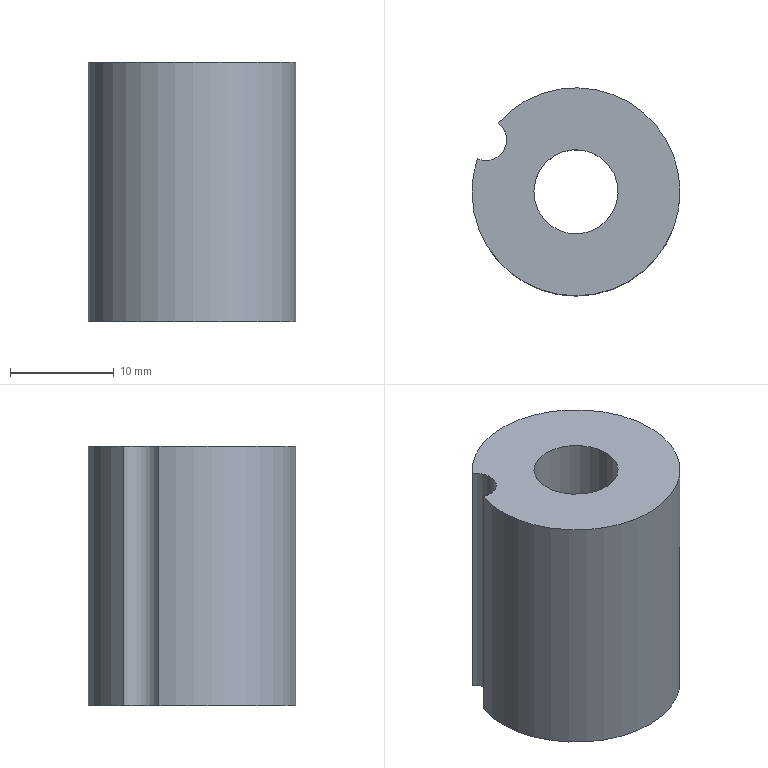Part | NX | features solid 2 | 1 solid | 7 faces | box 20 x 20 x 25 mm | volume 5172 mm3 | cylinder 4 | plane 3 | commonest cylinder face diameters 4 x1 8.1 x1 12.6 x1 20 x1
STEP:
#1=CARTESIAN_POINT('',(-312.495,434.194,24.));
#2=VERTEX_POINT('',#1);
#3=CARTESIAN_POINT('',(-312.495,434.194,49.));
#4=VERTEX_POINT('',#3);
#5=CARTESIAN_POINT('',(-312.495,434.194,36.5));
#6=DIRECTION('',(0.,0.,1.));
#7=VECTOR('',#6,1000.);
#8=LINE('',#5,#7);
#9=EDGE_CURVE('',#2,#4,#8,.T.);
#10=ORIENTED_EDGE('',*,*,#9,.T.);
#11=CARTESIAN_POINT('',(-314.485,430.747,49.));
#12=VERTEX_POINT('',#11);
#13=CARTESIAN_POINT('',(-305.003,427.57,49.));
#14=DIRECTION('',(0.,0.,-1.));
#15=DIRECTION('',(-0.866,0.5,0.));
#16=AXIS2_PLACEMENT_3D('',#13,#14,#15);
#17=CIRCLE('',#16,10.);
#18=EDGE_CURVE('',#4,#12,#17,.T.);
#19=ORIENTED_EDGE('',*,*,#18,.T.);
#20=CARTESIAN_POINT('',(-314.485,430.747,24.));
#21=VERTEX_POINT('',#20);
#22=CARTESIAN_POINT('',(-314.485,430.747,36.5));
#23=DIRECTION('',(0.,0.,1.));
#24=VECTOR('',#23,1000.);
#25=LINE('',#22,#24);
#26=EDGE_CURVE('',#12,#21,#25,.F.);
#27=ORIENTED_EDGE('',*,*,#26,.T.);
#28=CARTESIAN_POINT('',(-305.003,427.57,24.));
#29=DIRECTION('',(0.,0.,-1.));
#30=DIRECTION('',(-0.866,0.5,0.));
#31=AXIS2_PLACEMENT_3D('',#28,#29,#30);
#32=CIRCLE('',#31,10.);
#33=EDGE_CURVE('',#2,#21,#32,.T.);
#34=ORIENTED_EDGE('',*,*,#33,.F.);
#35=EDGE_LOOP('',(#10,#19,#27,#34));
#36=FACE_BOUND('',#35,.T.);
#37=CARTESIAN_POINT('',(-305.003,427.57,24.));
#38=DIRECTION('',(0.,0.,1.));
#39=DIRECTION('',(-0.866,0.5,0.));
#40=AXIS2_PLACEMENT_3D('',#37,#38,#39);
#41=CYLINDRICAL_SURFACE('',#40,10.);
#42=ADVANCED_FACE('',(#36),#41,.T.);
#43=CARTESIAN_POINT('',(-310.459,430.72,24.));
#44=VERTEX_POINT('',#43);
#45=CARTESIAN_POINT('',(-305.003,427.57,24.));
#46=DIRECTION('',(0.,0.,-1.));
#47=DIRECTION('',(-0.866,0.5,0.));
#48=AXIS2_PLACEMENT_3D('',#45,#46,#47);
#49=CIRCLE('',#48,6.3);
#50=EDGE_CURVE('',#44,#44,#49,.T.);
#51=ORIENTED_EDGE('',*,*,#50,.F.);
#52=EDGE_LOOP('',(#51));
#53=FACE_BOUND('',#52,.T.);
#54=ORIENTED_EDGE('',*,*,#33,.T.);
#55=CARTESIAN_POINT('',(-313.663,432.57,24.));
#56=DIRECTION('',(0.,0.,-1.));
#57=DIRECTION('',(-0.866,0.5,0.));
#58=AXIS2_PLACEMENT_3D('',#55,#56,#57);
#59=CIRCLE('',#58,2.);
#60=EDGE_CURVE('',#2,#21,#59,.T.);
#61=ORIENTED_EDGE('',*,*,#60,.F.);
#62=EDGE_LOOP('',(#54,#61));
#63=FACE_BOUND('',#62,.T.);
#64=CARTESIAN_POINT('',(-305.003,427.57,24.));
#65=DIRECTION('',(0.,0.,1.));
#66=DIRECTION('',(-0.866,0.5,0.));
#67=AXIS2_PLACEMENT_3D('',#64,#65,#66);
#68=PLANE('',#67);
#69=ADVANCED_FACE('',(#53,#63),#68,.F.);
#70=CARTESIAN_POINT('',(-308.51,429.595,49.));
#71=VERTEX_POINT('',#70);
#72=CARTESIAN_POINT('',(-305.003,427.57,49.));
#73=DIRECTION('',(0.,0.,-1.));
#74=DIRECTION('',(-0.866,0.5,0.));
#75=AXIS2_PLACEMENT_3D('',#72,#73,#74);
#76=CIRCLE('',#75,4.05);
#77=EDGE_CURVE('',#71,#71,#76,.T.);
#78=ORIENTED_EDGE('',*,*,#77,.T.);
#79=EDGE_LOOP('',(#78));
#80=FACE_BOUND('',#79,.T.);
#81=CARTESIAN_POINT('',(-313.663,432.57,49.));
#82=DIRECTION('',(0.,0.,-1.));
#83=DIRECTION('',(-0.866,0.5,0.));
#84=AXIS2_PLACEMENT_3D('',#81,#82,#83);
#85=CIRCLE('',#84,2.);
#86=EDGE_CURVE('',#4,#12,#85,.T.);
#87=ORIENTED_EDGE('',*,*,#86,.T.);
#88=ORIENTED_EDGE('',*,*,#18,.F.);
#89=EDGE_LOOP('',(#87,#88));
#90=FACE_BOUND('',#89,.T.);
#91=CARTESIAN_POINT('',(-305.003,427.57,49.));
#92=DIRECTION('',(0.,0.,1.));
#93=DIRECTION('',(-0.866,0.5,0.));
#94=AXIS2_PLACEMENT_3D('',#91,#92,#93);
#95=PLANE('',#94);
#96=ADVANCED_FACE('',(#80,#90),#95,.T.);
#97=ORIENTED_EDGE('',*,*,#50,.T.);
#98=EDGE_LOOP('',(#97));
#99=FACE_BOUND('',#98,.T.);
#100=CARTESIAN_POINT('',(-310.459,430.72,41.));
#101=VERTEX_POINT('',#100);
#102=CARTESIAN_POINT('',(-305.003,427.57,41.));
#103=DIRECTION('',(0.,0.,-1.));
#104=DIRECTION('',(-0.866,0.5,0.));
#105=AXIS2_PLACEMENT_3D('',#102,#103,#104);
#106=CIRCLE('',#105,6.3);
#107=EDGE_CURVE('',#101,#101,#106,.T.);
#108=ORIENTED_EDGE('',*,*,#107,.F.);
#109=EDGE_LOOP('',(#108));
#110=FACE_BOUND('',#109,.T.);
#111=CARTESIAN_POINT('',(-305.003,427.57,24.));
#112=DIRECTION('',(0.,0.,1.));
#113=DIRECTION('',(-0.866,0.5,0.));
#114=AXIS2_PLACEMENT_3D('',#111,#112,#113);
#115=CYLINDRICAL_SURFACE('',#114,6.3);
#116=ADVANCED_FACE('',(#99,#110),#115,.F.);
#117=CARTESIAN_POINT('',(-308.51,429.595,41.));
#118=VERTEX_POINT('',#117);
#119=CARTESIAN_POINT('',(-305.003,427.57,41.));
#120=DIRECTION('',(0.,0.,-1.));
#121=DIRECTION('',(-0.866,0.5,0.));
#122=AXIS2_PLACEMENT_3D('',#119,#120,#121);
#123=CIRCLE('',#122,4.05);
#124=EDGE_CURVE('',#118,#118,#123,.T.);
#125=ORIENTED_EDGE('',*,*,#124,.F.);
#126=EDGE_LOOP('',(#125));
#127=FACE_BOUND('',#126,.T.);
#128=ORIENTED_EDGE('',*,*,#107,.T.);
#129=EDGE_LOOP('',(#128));
#130=FACE_BOUND('',#129,.T.);
#131=CARTESIAN_POINT('',(-305.003,427.57,41.));
#132=DIRECTION('',(0.,0.,1.));
#133=DIRECTION('',(-0.866,0.5,0.));
#134=AXIS2_PLACEMENT_3D('',#131,#132,#133);
#135=PLANE('',#134);
#136=ADVANCED_FACE('',(#127,#130),#135,.F.);
#137=ORIENTED_EDGE('',*,*,#9,.F.);
#138=ORIENTED_EDGE('',*,*,#60,.T.);
#139=ORIENTED_EDGE('',*,*,#26,.F.);
#140=ORIENTED_EDGE('',*,*,#86,.F.);
#141=EDGE_LOOP('',(#137,#138,#139,#140));
#142=FACE_BOUND('',#141,.T.);
#143=CARTESIAN_POINT('',(-313.663,432.57,24.));
#144=DIRECTION('',(0.,0.,1.));
#145=DIRECTION('',(-0.866,0.5,0.));
#146=AXIS2_PLACEMENT_3D('',#143,#144,#145);
#147=CYLINDRICAL_SURFACE('',#146,2.);
#148=ADVANCED_FACE('',(#142),#147,.F.);
#149=ORIENTED_EDGE('',*,*,#77,.F.);
#150=EDGE_LOOP('',(#149));
#151=FACE_BOUND('',#150,.T.);
#152=ORIENTED_EDGE('',*,*,#124,.T.);
#153=EDGE_LOOP('',(#152));
#154=FACE_BOUND('',#153,.T.);
#155=CARTESIAN_POINT('',(-305.003,427.57,24.));
#156=DIRECTION('',(0.,0.,1.));
#157=DIRECTION('',(-0.866,0.5,0.));
#158=AXIS2_PLACEMENT_3D('',#155,#156,#157);
#159=CYLINDRICAL_SURFACE('',#158,4.05);
#160=ADVANCED_FACE('',(#151,#154),#159,.F.);
#161=CLOSED_SHELL('',(#42,#69,#96,#116,#136,#148,#160));
#162=MANIFOLD_SOLID_BREP('',#161);
#163=(LENGTH_UNIT()NAMED_UNIT(*)SI_UNIT(.MILLI.,.METRE.));
#164=UNCERTAINTY_MEASURE_WITH_UNIT(LENGTH_MEASURE(0.00001),#163,'','');
#165=(NAMED_UNIT(*)PLANE_ANGLE_UNIT()SI_UNIT($,.RADIAN.));
#166=(NAMED_UNIT(*)SI_UNIT($,.STERADIAN.)SOLID_ANGLE_UNIT());
#167=(GEOMETRIC_REPRESENTATION_CONTEXT(3)GLOBAL_UNCERTAINTY_ASSIGNED_CONTEXT((#164))GLOBAL_UNIT_ASSIGNED_CONTEXT((#163,#165,#166))REPRESENTATION_CONTEXT('',''));
#168=ADVANCED_BREP_SHAPE_REPRESENTATION('',(#162),#167);